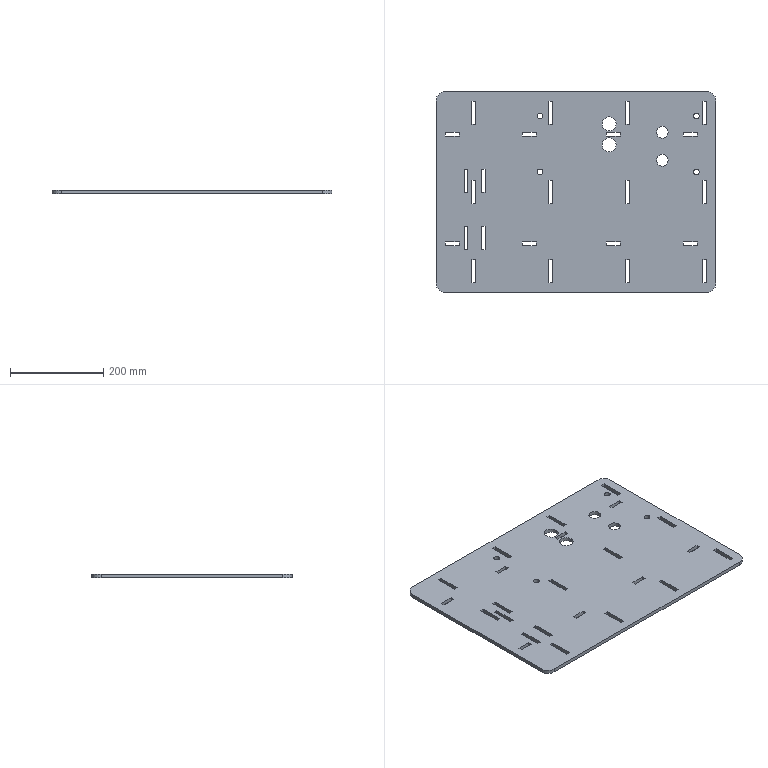Part | SolidWorks | features FlatPattern 1, SMBaseFlange 1, SheetMetal 1 | 1 solid | 122 faces | box 600 x 430 x 8 mm | volume 1971602 mm3 | plane 102 | cylinder 20 | commonest cylinder face diameters 12.5 x8 25 x4 30 x4 40 x4